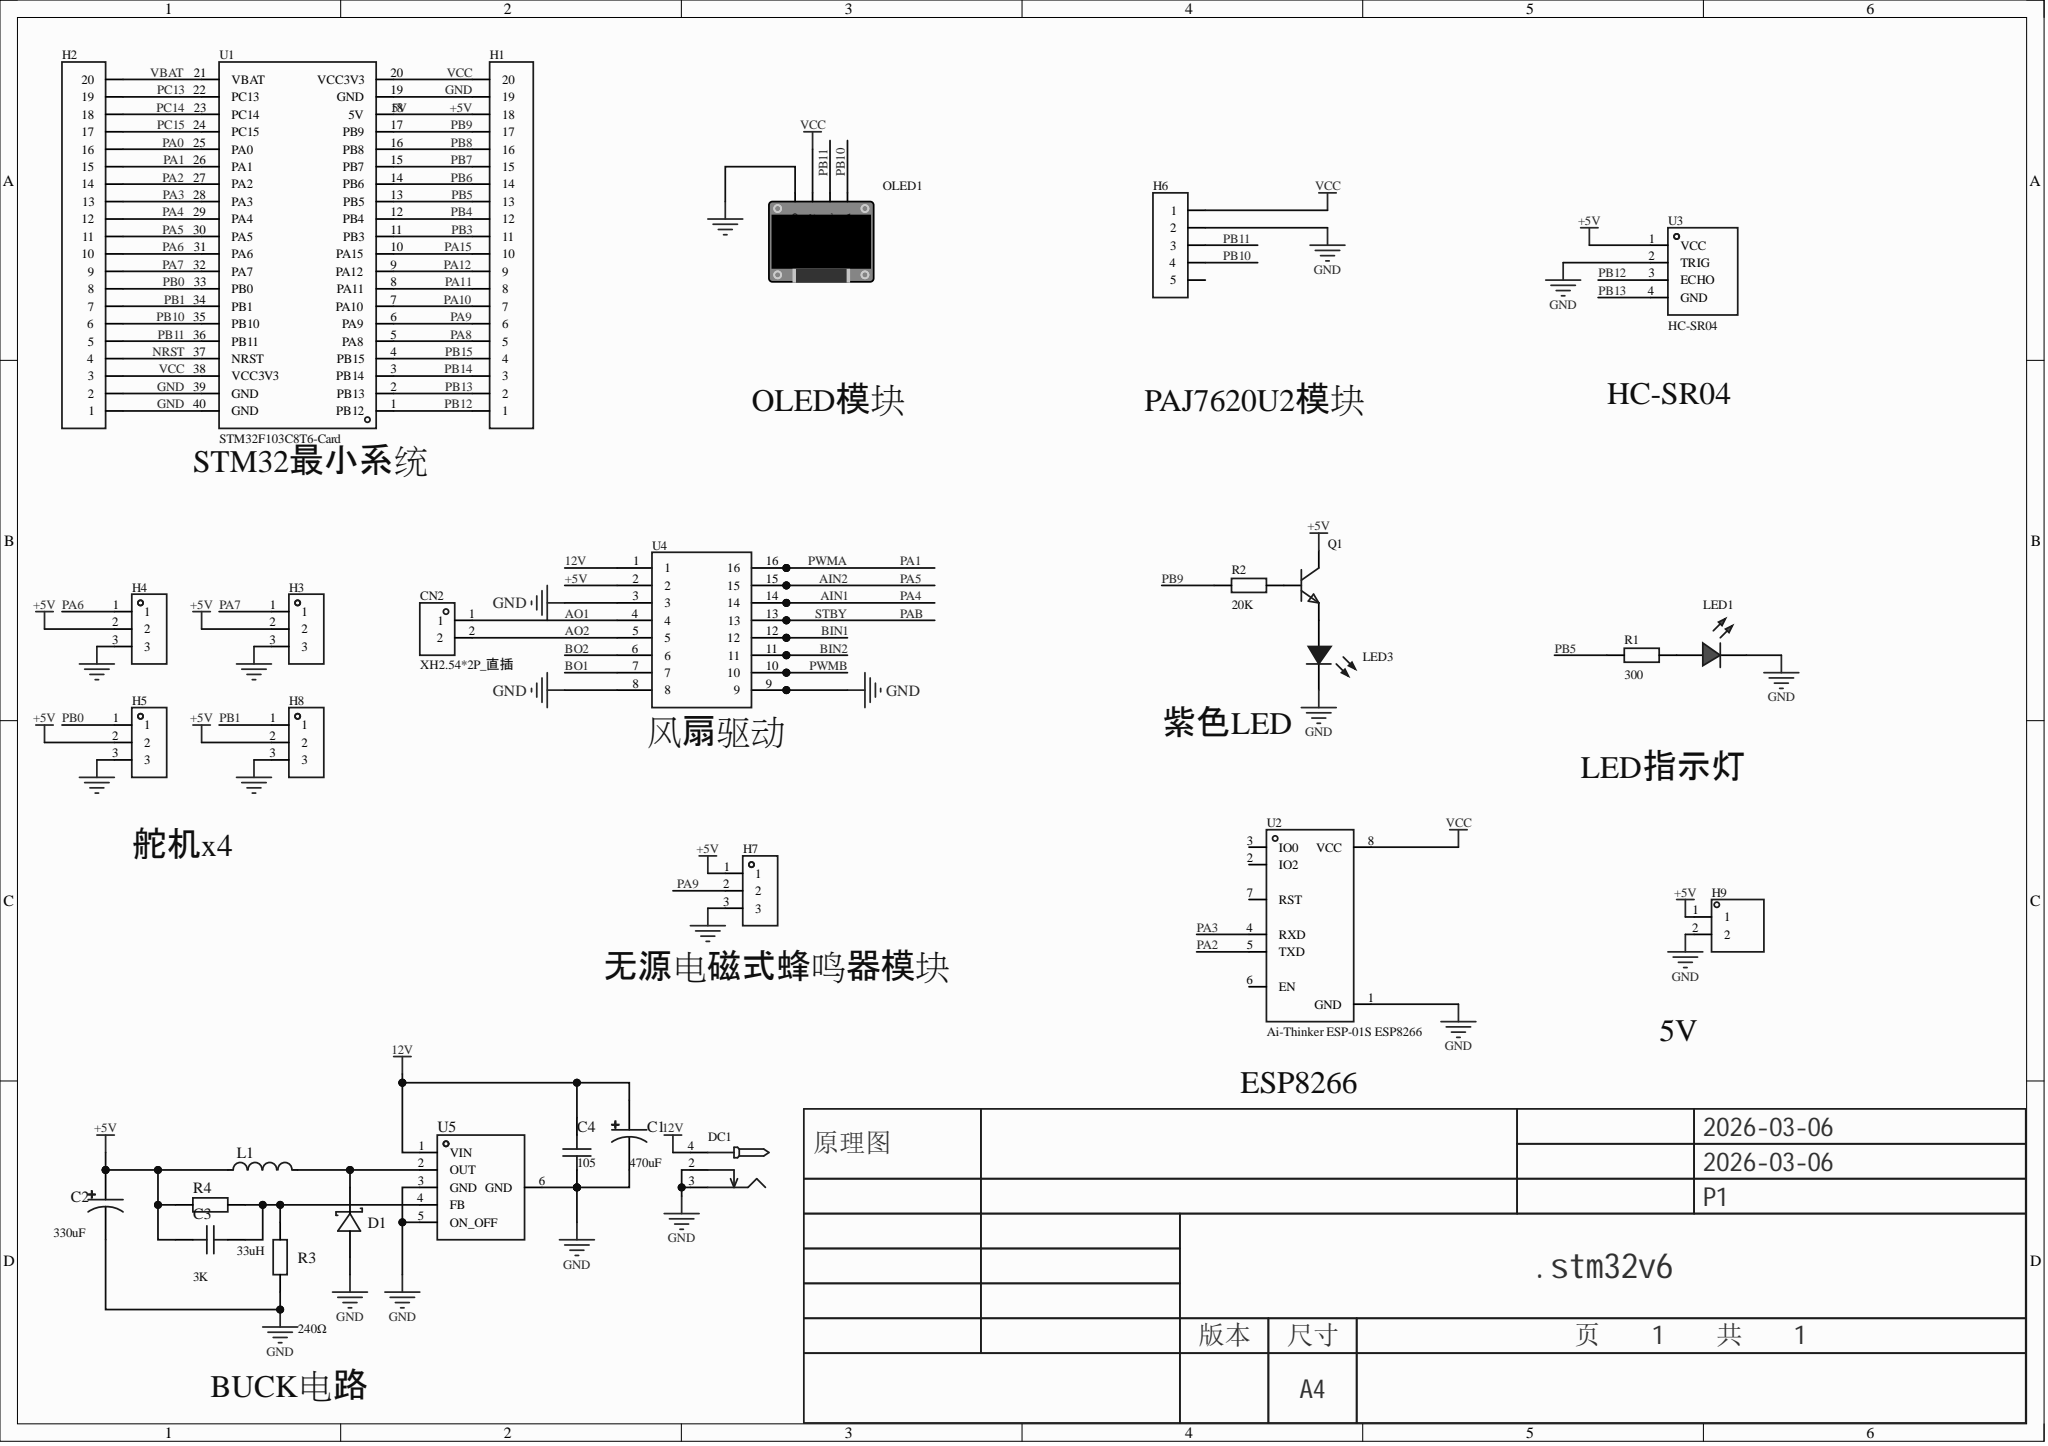Circuit board | Altium Designer | 30 parts | 45 nets
Bill of materials:
Comment,Description,Designator,Footprint,LibRef,Quantity
"","","C1, C2","CAP-SMD_BD8.0-L8.3-W8.3-LS9.0-FD","OCV471M0JTR-0812","2"
"","额定电压:6.3V;容值:22uF;温度系数:X5R;精度:±20%;","C3, C4","C0603","C0603X5R226M6R3NT","2"
"XH2.54*2P_直插","","CN2","CONN-TH_2P-P2.50-XH2.54-2P","XH2.54*2P_直插","1"
"","直流反向耐压(Vr):40V;正向压降(Vf):550mV 3A;平均整流电流(Io):3A;","D1","SMA_L4.4-W2.6-LS5.0-RD","SS34A_C183891","1"
"","","DC1","DC-2.0","DC-005_2.0","1"
"","","H1, H2","HDR-TH_20P-P2.54-V-F","HDR-F_2.54_1x20P","2"
"","","H3, H4, H5, H7, H8","HDR-TH_3P-P2.54-V-F","HDR-F_2.54_1x3P","5"
"","","H6","HDR-TH_5P-P2.54-V-F","HDR-F_2.54_1x5P","1"
"","","H9","HDR-TH_2P-P2.54-V-M-1","HDR-M_2.54_1x2P","1"
"","","L1","IND-SMD_L13.5-W12.6","FXL1350-470-M","1"
"","","LED1, LED3","LED-TH_5mm","LED_TH-R_5mm, LED_TH-B_5mm","2"
"","","OLED1","0.96OLED_4P","0.96OLED模块_4P","1"
"","","Q1","S8050_SOT-23","S8050_SOT_NPN","1"
"300","","R1","R0603","Res_0603","1"
"20K","","R2","R0603","Res_0603","1"
"","","R3, R4","R0603","RCT03240RFLF","2"
"STM32F103C8T6-Card","","U1","CONN-TH_L53.3-W22.9_STM32F103C8T6-CARD","STM32F103C8T6-Card","1"
"Ai-Thinker ESP-01S ESP8266","","U2","WIFIM-TH_8P-L24.7-W14.4-P2.54","Ai-Thinker ESP-01S ESP8266","1"
"HC-SR04","","U3","TH_HC-SR04V","HC-SR04","1"
"","","U4","tb6612","tb6612","1"
"","","U5","TO-263-5_L10.2-W8.9-P1.70-BR","LM2596S-ADJ/TR_C918142","1"
Netlist (Protel format):
[
C1
CAP-SMD_BD8.0-L8.3-W8.3-LS9.0-FD




]
[
C2
CAP-SMD_BD8.0-L8.3-W8.3-LS9.0-FD




]
[
C3
C0603




]
[
C4
C0603




]
[
CN2
CONN-TH_2P-P2.50-XH2.54-2P
XH2.54*2P_直插



]
[
D1
SMA_L4.4-W2.6-LS5.0-RD




]
[
DC1
DC-2.0




]
[
H1
HDR-TH_20P-P2.54-V-F




]
[
H2
HDR-TH_20P-P2.54-V-F




]
[
H3
HDR-TH_3P-P2.54-V-F




]
[
H4
HDR-TH_3P-P2.54-V-F




]
[
H5
HDR-TH_3P-P2.54-V-F




]
[
H6
HDR-TH_5P-P2.54-V-F




]
[
H7
HDR-TH_3P-P2.54-V-F




]
[
H8
HDR-TH_3P-P2.54-V-F




]
[
H9
HDR-TH_2P-P2.54-V-M-1




]
[
L1
IND-SMD_L13.5-W12.6




]
[
LED1
LED-TH_5mm




]
[
LED3
LED-TH_5mm




]
[
OLED1
0.96OLED_4P




]
[
Q1
S8050_SOT-23




]
[
R1
R0603
300



]
[
R2
R0603
20K



]
[
R3
R0603




]
[
R4
R0603




]
[
U1
CONN-TH_L53.3-W22.9_STM32F103C8T6-CARD
STM32F103C8T6-Card



]
[
U2
WIFIM-TH_8P-L24.7-W14.4-P2.54
Ai-Thinker ESP-01S ESP8266



]
[
U3
TH_HC-SR04V
HC-SR04



]
[
U4
tb6612




]
[
U5
TO-263-5_L10.2-W8.9-P1.70-BR




]
(
VCC
H1-20
H2-3
H6-1
OLED1-2
U1-20
U1-38
U2-8
)
(
VBAT
H2-20
U1-21
)
(
PC15
H2-17
U1-24
)
(
PC14
H2-18
U1-23
)
(
PC13
H2-19
U1-22
)
(
PB15
H1-4
U1-4
)
(
PB14
H1-3
U1-3
)
(
PB13
H1-2
U1-2
U3-4
)
(
PB12
H1-1
U1-1
U3-3
)
(
PB11
H2-5
H6-3
OLED1-3
U1-36
)
(
PB10
H2-6
H6-4
OLED1-4
U1-35
)
(
PB9
H1-17
R2-1
U1-17
)
(
PB8
H1-16
U1-16
)
(
PB7
H1-15
U1-15
)
(
PB6
H1-14
U1-14
)
(
PB5
H1-13
R1-2
U1-13
)
(
PB4
H1-12
U1-12
)
(
PB3
H1-11
U1-11
)
(
PB1
H2-7
H8-1
U1-34
)
(
PB0
H2-8
H5-1
U1-33
)
(
PA15
H1-10
U1-10
)
(
PA12
H1-9
U1-9
)
(
PA11
H1-8
U1-8
)
(
PA10
H1-7
U1-7
)
(
PA9
H1-6
H7-2
U1-6
)
(
PA8
H1-5
U1-5
)
(
PA7
H2-9
H3-1
U1-32
)
(
PA6
H2-10
H4-1
U1-31
)
(
PA3
H2-13
U1-28
U2-4
)
(
PA2
H2-14
U1-27
U2-5
)
(
PA1
H2-15
U1-26
U4-16
)
(
PA0
H2-16
U1-25
)
(
NRST
H2-4
U1-37
)
(
NetQ1_1
Q1-1
R2-2
)
(
NetLED3_1
LED3-1
Q1-2
)
(
NetLED1_1
LED1-1
R1-1
)
(
NetD1_1
D1-1
L1-2
U5-2
)
(
NetC3_2
C3-2
R3-1
R4-2
U5-4
)
(
GND
C1-2
C2-2
C4-2
D1-2
DC1-2
DC1-3
H1-19
H2-1
H2-2
H3-3
H4-3
H5-3
H6-2
H7-3
H8-3
H9-2
LED1-2
LED3-2
OLED1-1
R3-2
U1-19
U1-39
U1-40
U2-1
U3-2
U4-3
U4-8
U4-9
U5-3
U5-5
U5-6
)
(
AO2
CN2-2
U4-5
)
(
AO1
CN2-1
U4-4
)
(
AIN2
H2-11
U1-30
U4-15
)
(
AIN1
H2-12
U1-29
U4-14
)
(
12V
C1-1
C4-1
DC1-4
U4-1
U5-1
)
(
5V
C2-1
C3-1
H1-18
H3-2
H4-2
H5-2
H7-1
H8-2
H9-1
L1-1
Q1-3
R4-1
U1-18
U3-1
U4-2
)